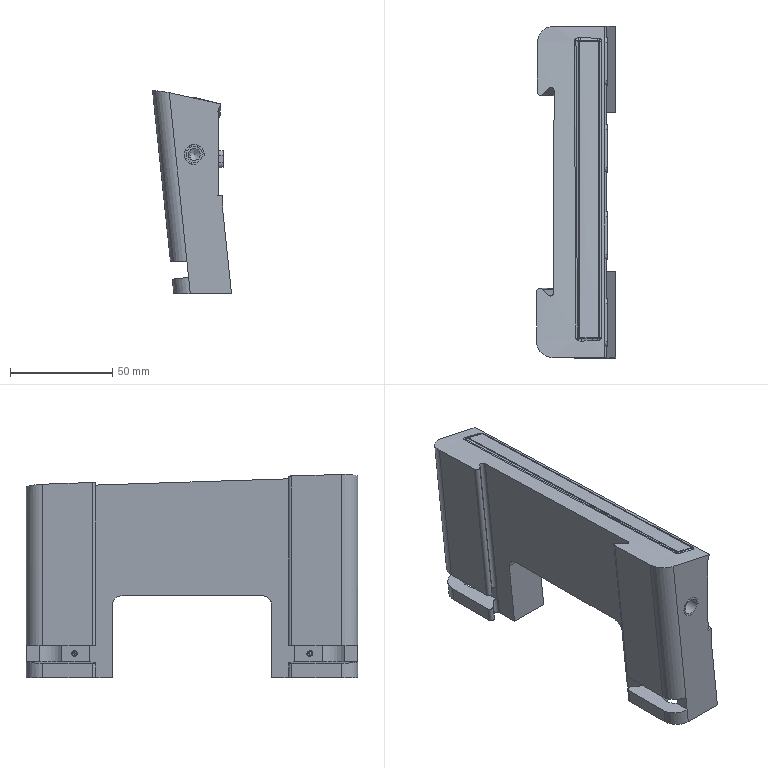Part | STEP file | P011002L002-000 | 1 solid | 254 faces | box 38.575 x 161.92 x 99.169 mm | volume 274542 mm3 | plane 117 | cylinder 44 | spline 33 | other 29 | cone 27 | sphere 4 | commonest cylinder face diameters 5 x16 3 x10 16 x6 6 x3 2.5 x2 2.99 x2